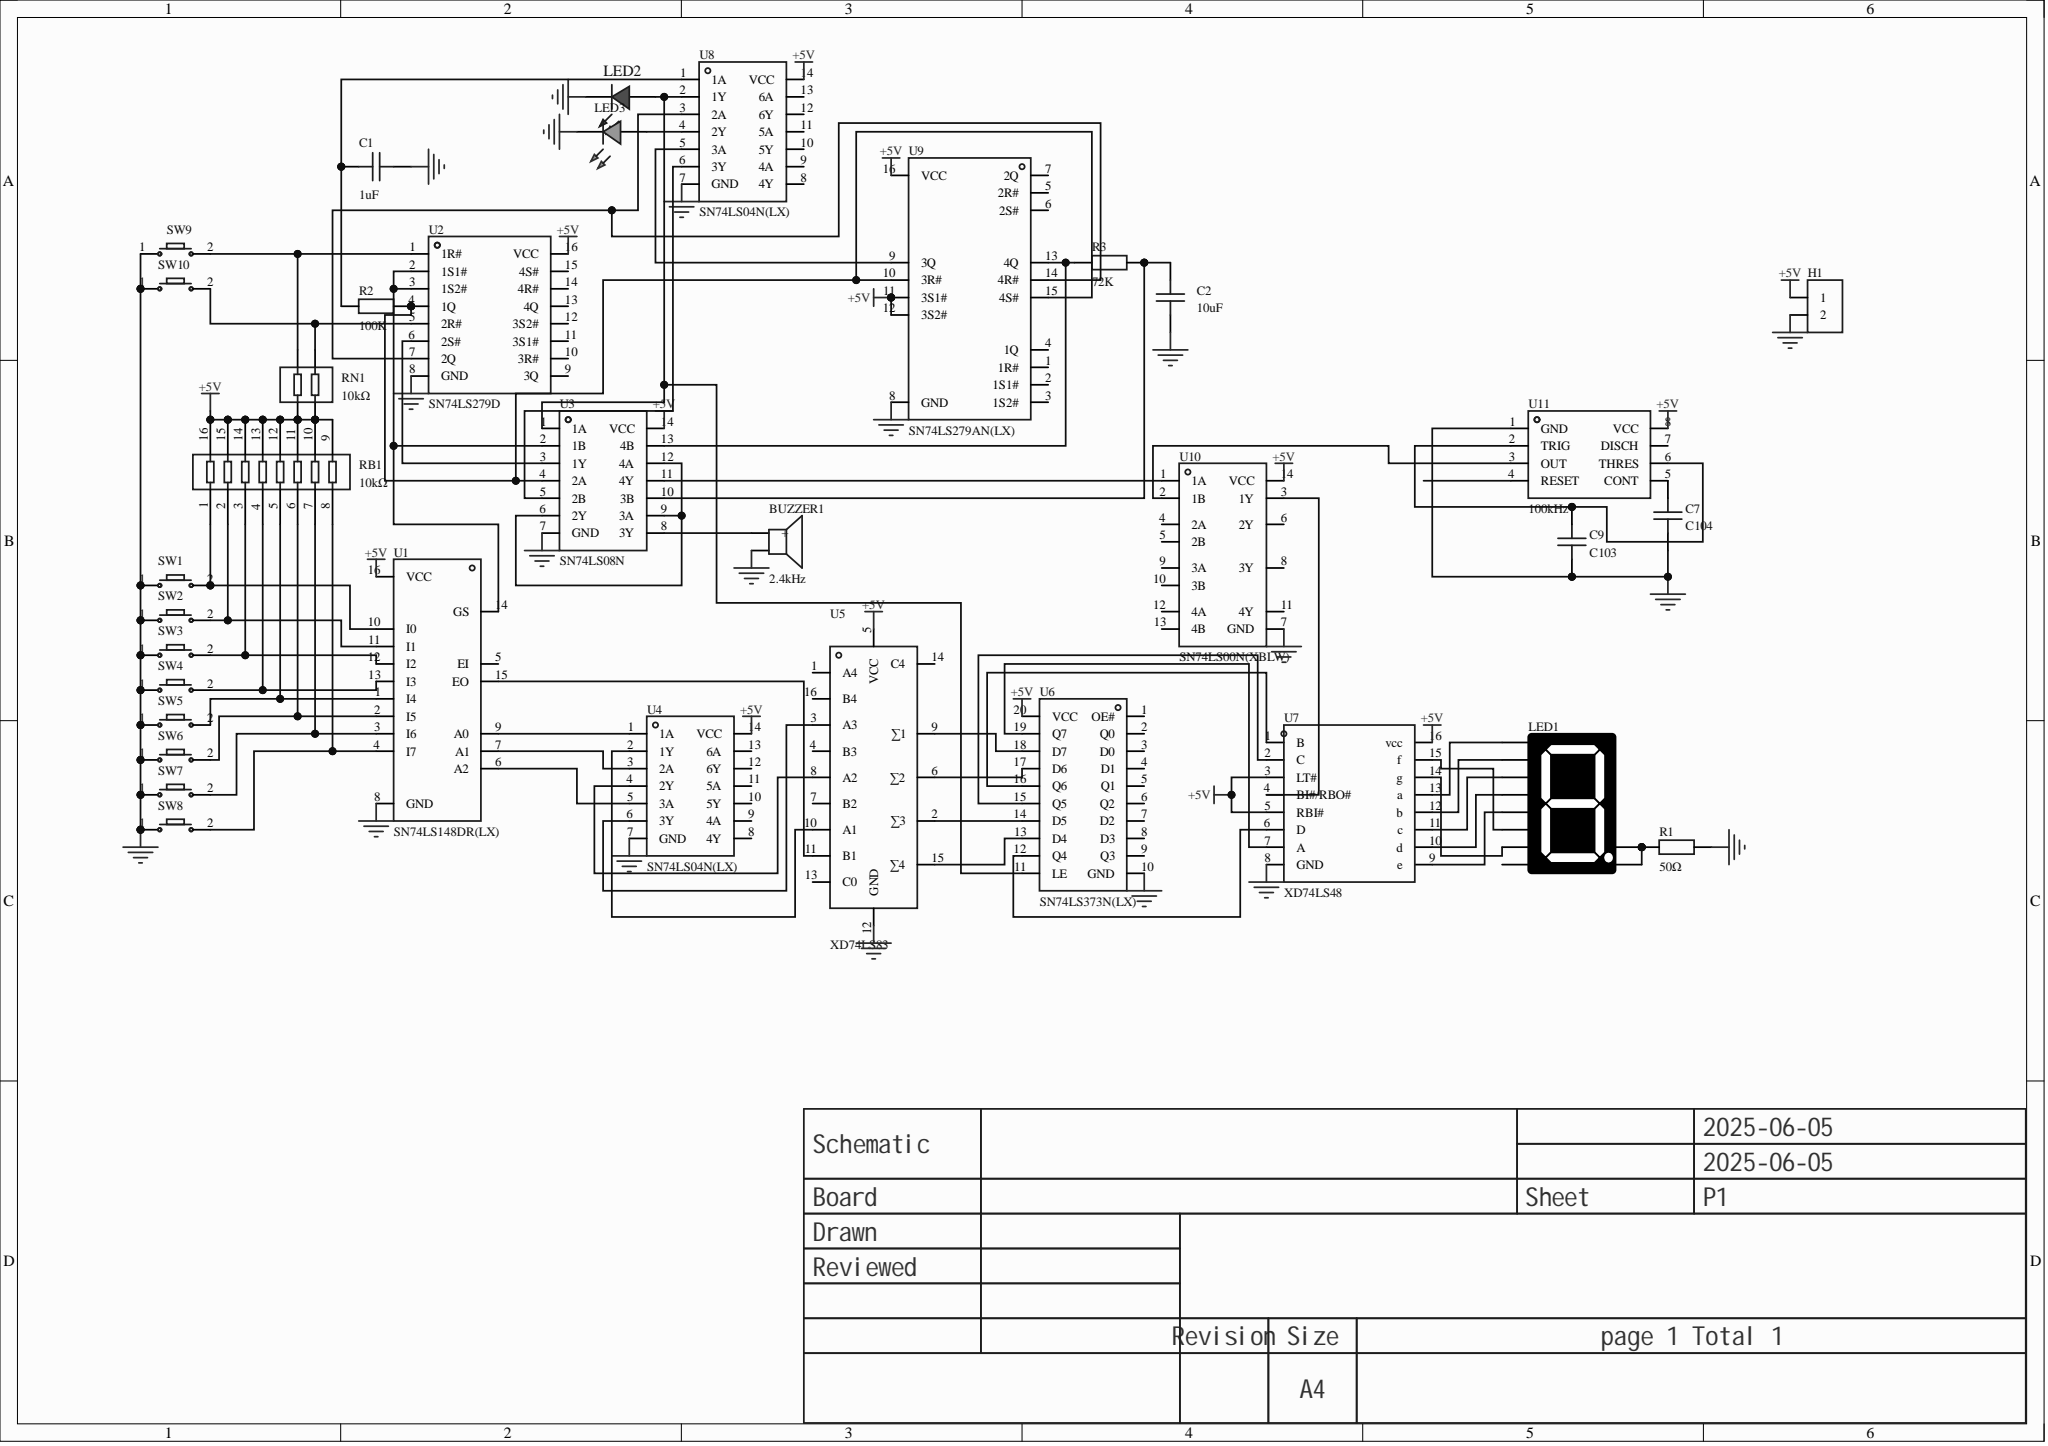Circuit board | Altium Designer | 35 parts | 53 nets
Bill of materials:
Comment,Description,Designator,Footprint,LibRef,Quantity
"2.4kHz","Drive mode:Active (built-in driver); Construction:Electromagnetic; Rated voltage:-; Frequency:2.4kHz; Sound pressure (SPL):85dB;","BUZZER1","BUZ-TH_BD12.0-P7.60-D0.6-FD","TMB12A05_C96093","1"
"1uF","","C1","C0603","CAP_0603","1"
"10uF","","C2","C0603","CAP_0603","1"
"C104","Capacitance:100nF; Tolerance:±10%; Rated voltage:50V; Temp coefficient:X7R;","C7","CAP-TH_L8.5-W5.0-P5.00-D1.2","CT4-0805B104K500F3","1"
"C103","Capacitance:100nF; Tolerance:±10%; Rated voltage:50V; Temp coefficient:X7R;","C9","CAP-TH_L8.5-W5.0-P5.00-D1.2","CT4-0805B104K500F3","1"
"","","H1","HDR-TH_2P-P2.54-V-F","HDR-F_2.54_1x2P","1"
"","","LED1","LED-SEG-TH_10P-L12.6-W19.0-P2.54-S15.24-BL","LED_SEG_TH_0.56x1","1"
"","","LED2, LED3","LED_0805","LED_0805-R, LED_0805-G","2"
"50Ω","","R1","R0603","Res_0603","1"
"100K","","R2","R0805","Res_0805","1"
"72K","","R3","R0805","Res_0805","1"
"10kΩ","Resistor count:8; Resistance:10kΩ; Tolerance:±5%; Power per element:63mW; Temp coefficient:±200ppm/?;","RB1","RES-ARRAY-SMD_0603-16P-L6.4-W1.6-TL","742C163103JP","1"
"10kΩ","Resistor count:2; Resistance:10kΩ; Tolerance:±5%; Power per element:62.5mW; Temp coefficient:±200ppm/?;","RN1","RES-ARRAY-SMD_0603-4P-L1.6-W1.6-BL","2D03WGJ0103T5E","1"
"","","SW1, SW2, SW3, SW4, SW5, SW6, SW7, SW8, SW9, SW10","Key_SMD_3x4x2","Key_SMD_3x4x2","10"
"SN74LS148DR(LX)","","U1","SOIC-16_L9.9-W3.9-P1.27-LS6.0-BL-1","SN74LS148DR(LX)","1"
"SN74LS279D","","U2","SOIC-16_L9.9-W3.9-P1.27-LS6.0-BL","SN74LS279D","1"
"SN74LS08N","Logic type:AND gate; Channels:4; Operating voltage:4.75V~5.25V; Propagation delay (tpd):-;","U3","PDIP-14_L19.3-W6.4-P2.54-LS7.9-BL-1","SN74LS08N","1"
"SN74LS04N(LX)","Operating voltage:2V~6V; Operating current:2uA; Channels:6; Propagation delay (tpd):14ns@6V;","U4, U8","DIP-14_L19.1-W6.4-P2.54-LS7.6-BL","SN74LS04N(LX)","2"
"XD74LS83","Channels:2; Operating voltage:5V;","U5","PDIP-16_L19.1-W6.4-P2.54-LS7.62-BL","XD74LS83","1"
"SN74LS373N(LX)","Logic type:D-type latch; Operating voltage:2V~6V; Channels:8; Propagation delay (tpd):26ns;","U6","PDIP-20_L26.2-W7.6-P2.54-LS7.9-BL","SN74LS373N(LX)","1"
"XD74LS48","Decoder/driver, 4-to-7","U7","DIP-16_L19.3-W6.4-P2.54-LS7.6-BL","XD74LS48","1"
"SN74LS279AN(LX)","Logic type:S-R latch; Supply voltage:2V~6V; Channels:4; Propagation delay:33ns;","U9","PDIP-16_L19.3-W6.4-P2.54-LS7.94-BL","SN74LS279AN(LX)","1"
"SN74LS00N(XBLW)","SN74LS00 is a quad 2-input NAND gate; inputs include clamp diodes, allowing a current-limiting resistor to connect the input to a voltage above Vcc.","U10","PDIP-14_L19.3-W6.4-P2.54-LS7.6-BL","SN74LS00N(XBLW)","1"
"100kHz","Frequency:100kHz;","U11","DIP-8_L9.8-W6.6-P2.54-LS7.6-BL","NE555P","1"
Netlist (Protel format):
[
BUZZER1
BUZ-TH_BD12.0-P7.60-D0.6-FD
2.4kHz



]
[
C1
C0603
1uF



]
[
C2
C0603
10uF



]
[
C7
CAP-TH_L8.5-W5.0-P5.00-D1.2
C104



]
[
C9
CAP-TH_L8.5-W5.0-P5.00-D1.2
C103



]
[
H1
HDR-TH_2P-P2.54-V-F




]
[
LED1
LED-SEG-TH_10P-L12.6-W19.0-P2.54-S15.24-BL




]
[
LED2
LED_0805




]
[
LED3
LED_0805




]
[
R1
R0603
50Ω



]
[
R2
R0805
100K



]
[
R3
R0805
72K



]
[
RB1
RES-ARRAY-SMD_0603-16P-L6.4-W1.6-TL
10kΩ



]
[
RN1
RES-ARRAY-SMD_0603-4P-L1.6-W1.6-BL
10kΩ



]
[
SW1
Key_SMD_3x4x2




]
[
SW2
Key_SMD_3x4x2




]
[
SW3
Key_SMD_3x4x2




]
[
SW4
Key_SMD_3x4x2




]
[
SW5
Key_SMD_3x4x2




]
[
SW6
Key_SMD_3x4x2




]
[
SW7
Key_SMD_3x4x2




]
[
SW8
Key_SMD_3x4x2




]
[
SW9
Key_SMD_3x4x2




]
[
SW10
Key_SMD_3x4x2




]
[
U1
SOIC-16_L9.9-W3.9-P1.27-LS6.0-BL-1
SN74LS148DR(LX)



]
[
U2
SOIC-16_L9.9-W3.9-P1.27-LS6.0-BL
SN74LS279D



]
[
U3
PDIP-14_L19.3-W6.4-P2.54-LS7.9-BL-1
SN74LS08N



]
[
U4
DIP-14_L19.1-W6.4-P2.54-LS7.6-BL
SN74LS04N(LX)



]
[
U5
PDIP-16_L19.1-W6.4-P2.54-LS7.62-BL
XD74LS83



]
[
U6
PDIP-20_L26.2-W7.6-P2.54-LS7.9-BL
SN74LS373N(LX)



]
[
U7
DIP-16_L19.3-W6.4-P2.54-LS7.6-BL
XD74LS48



]
[
U8
DIP-14_L19.1-W6.4-P2.54-LS7.6-BL
SN74LS04N(LX)



]
[
U9
PDIP-16_L19.3-W6.4-P2.54-LS7.94-BL
SN74LS279AN(LX)



]
[
U10
PDIP-14_L19.3-W6.4-P2.54-LS7.6-BL
SN74LS00N(XBLW)



]
[
U11
DIP-8_L9.8-W6.6-P2.54-LS7.6-BL
100kHz



]
(
NetU10_2
U10-2
U11-3
)
(
NetU8_5
U8-5
U9-9
)
(
NetU7_4
U7-4
U10-3
)
(
NetU6_19
U6-19
U7-7
)
(
NetU6_16
U6-16
U7-1
)
(
NetU6_15
U6-15
U7-2
)
(
NetU6_12
U6-12
U7-6
)
(
NetU5_15
U5-15
U6-13
)
(
NetU5_9
U5-9
U6-18
)
(
NetU5_6
U5-6
U6-17
)
(
NetU5_2
U5-2
U6-14
)
(
NetU4_6
U4-6
U5-3
)
(
NetU4_4
U4-4
U5-8
)
(
NetU4_2
U4-2
U5-10
)
(
NetU3_11
U3-11
U10-1
)
(
NetU3_6
U3-6
U3-9
U3-12
)
(
NetU3_5
U3-5
U8-6
)
(
NetU2_7
U2-7
U8-3
U9-14
)
(
NetU2_6
U2-6
U3-3
)
(
NetU1_15
U1-15
U5-11
)
(
NetU1_14
U1-14
U2-2
U2-3
U3-2
)
(
NetU1_9
U1-9
U4-1
)
(
NetU1_7
U1-7
U4-3
)
(
NetU1_6
U1-6
U4-5
)
(
NetRN1_4
RN1-4
SW9-2
U2-1
)
(
NetRN1_3
RN1-3
SW10-2
U2-5
)
(
NetRB1_8
RB1-8
SW8-2
U1-4
)
(
NetRB1_7
RB1-7
SW7-2
U1-3
)
(
NetRB1_6
RB1-6
SW6-2
U1-2
)
(
NetRB1_5
RB1-5
SW5-2
U1-1
)
(
NetRB1_4
RB1-4
SW4-2
U1-13
)
(
NetRB1_3
RB1-3
SW3-2
U1-12
)
(
NetRB1_2
RB1-2
SW2-2
U1-11
)
(
NetRB1_1
RB1-1
SW1-2
U1-10
)
(
NetR3_1
R3-1
U3-13
U9-13
)
(
NetR2_2
R2-2
U2-4
U3-4
U9-10
U9-15
)
(
NetLED3_2
LED3-2
U8-4
)
(
NetLED2_2
LED2-2
U3-1
U6-11
U8-2
)
(
NetLED1_10
LED1-10
U7-14
)
(
NetLED1_9
LED1-9
U7-15
)
(
NetLED1_7
LED1-7
U7-13
)
(
NetLED1_6
LED1-6
U7-12
)
(
NetLED1_4
LED1-4
U7-11
)
(
NetLED1_3
LED1-3
LED1-8
R1-2
)
(
NetLED1_2
LED1-2
U7-10
)
(
NetLED1_1
LED1-1
U7-9
)
(
NetC9_2
C9-2
U11-2
U11-6
)
(
NetC7_2
C7-2
U11-5
)
(
NetC2_2
C2-2
R3-2
U3-10
)
(
NetC1_1
C1-1
R2-1
U8-1
)
(
NetBUZZER1_1
BUZZER1-1
U3-8
)
(
GND
BUZZER1-2
C1-2
C2-1
C7-1
C9-1
H1-2
LED2-1
LED3-1
R1-1
SW1-1
SW2-1
SW3-1
SW4-1
SW5-1
SW6-1
SW7-1
SW8-1
SW9-1
SW10-1
U1-8
U2-8
U3-7
U4-7
U5-12
U6-10
U7-8
U8-7
U9-8
U10-7
U11-1
)
(
+5V
H1-1
RB1-9
RB1-10
RB1-11
RB1-12
RB1-13
RB1-14
RB1-15
RB1-16
RN1-1
RN1-2
U1-16
U2-16
U3-14
U4-14
U5-5
U6-20
U7-3
U7-5
U7-16
U8-14
U9-11
U9-12
U9-16
U10-14
U11-8
)